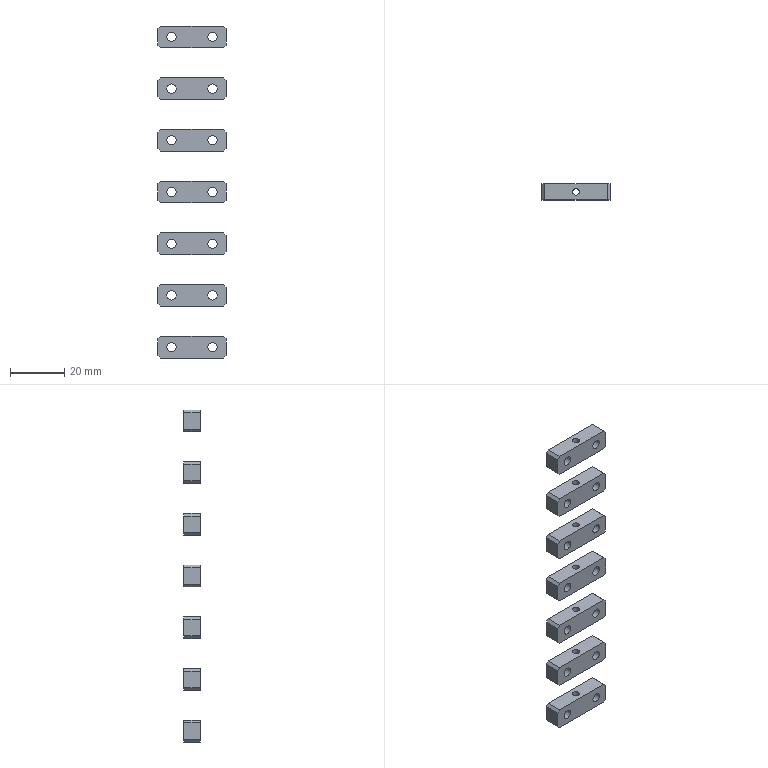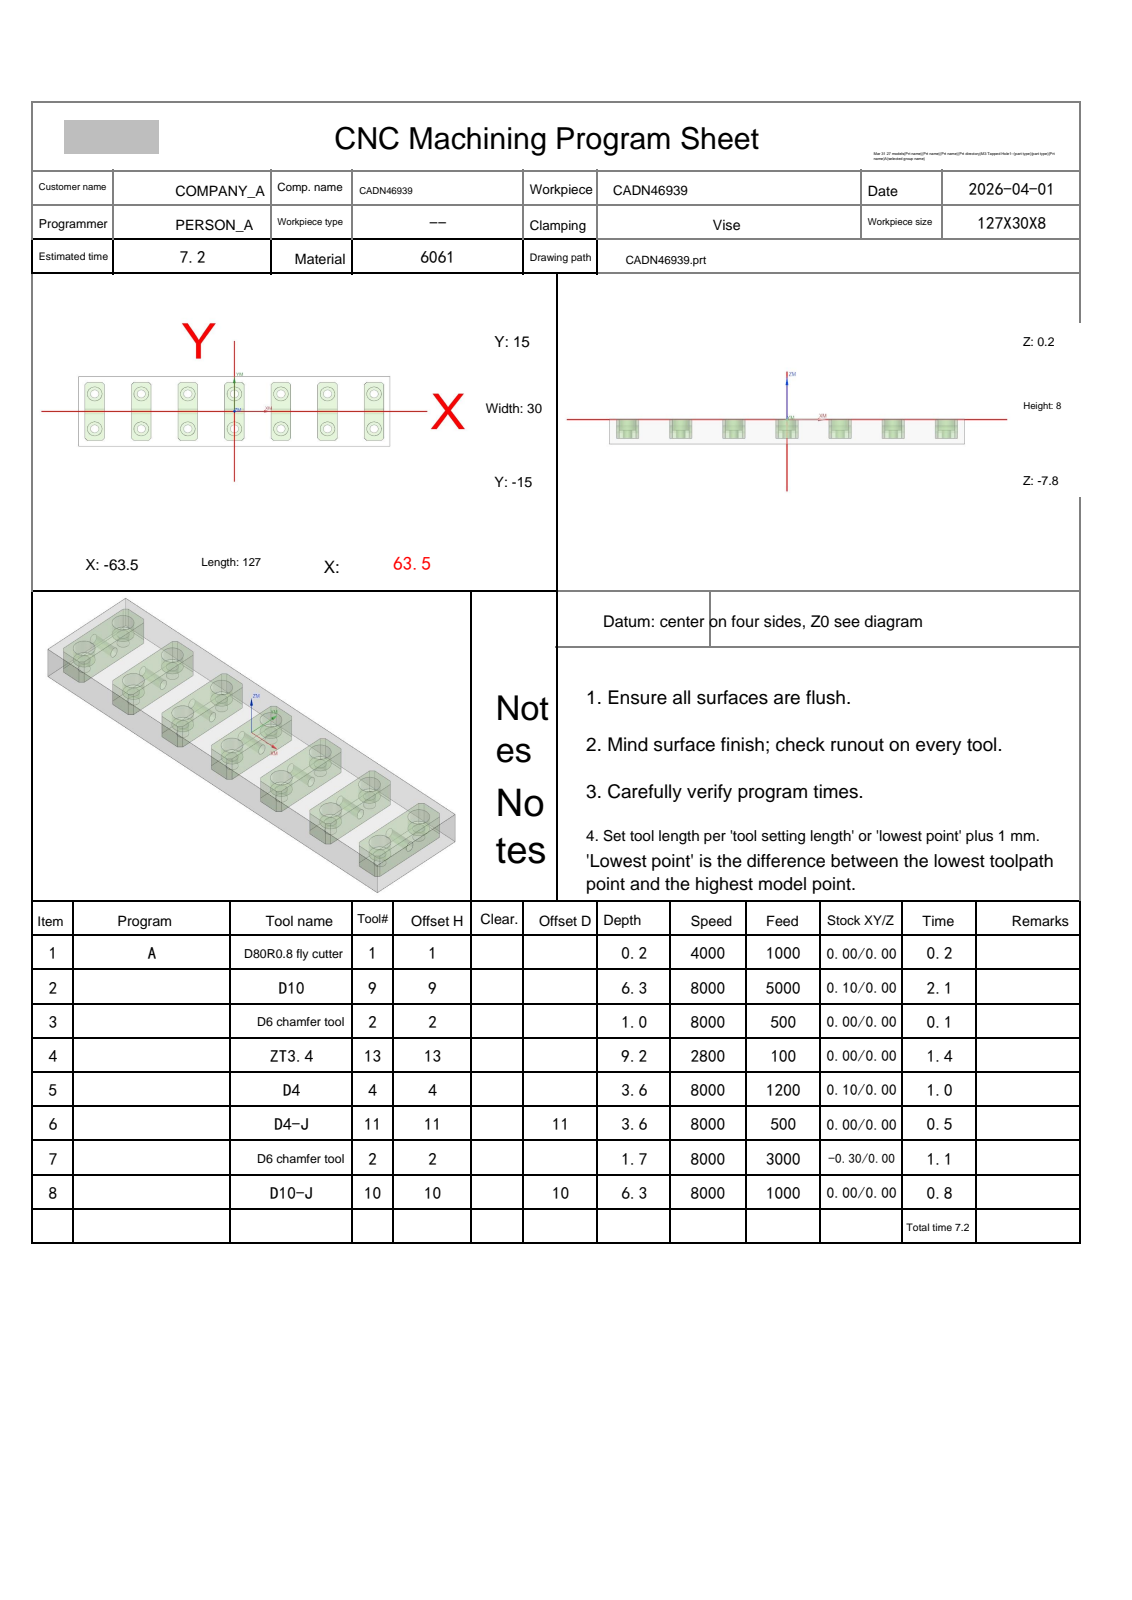NC program | NX | posted by the shop | part box 25 x 6 x 122 mm
Lines 1772 to 3537 of 3537, first 1667 of 1766 lines:
N3 T02 M06
(D6 chamfer tool  D=6. R=0. H=02 ce=0.00 di=0.00)
G00 G90 G54 X-57. Y7.5 M03 S8000
G43 H02 Z20.
M08
G98 G81 X-57. Y7.5 Z-.8 R1. F500.
Y-7.5
X-38.
Y7.5
X-19.
Y-7.5
X0.0
Y7.5
X19.
Y-7.5
X38.
Y7.5
X57.
Y-7.5
G80
G00 Z20.
G91 G28 Z0.0
M05
M09
G91 G28 Z0.0
M01
N4 T13 M06
(ZT3.4 D=3.4 DR_a=118 H=13)
G00 G90 G54 X-57. Y7.5 M03 S2800
G43 H13 Z20.
M08
G98 G83 X-57. Y7.5 Z-9.021 R1. F100. Q2.
Y-7.5
X-38.
Y7.5
X-19.
Y-7.5
X0.0
Y7.5
X19.
Y-7.5
X38.
Y7.5
X57.
Y-7.5
G80
G00 Z20.
G91 G28 Z0.0
M05
M09
G91 G28 Z0.0
M01
N5 T04 M06
(D4  D=4. R=0. H=04 ce=0.10 di=0.00)
G00 G90 G54 X-57. Y7.5 M03 S8000
G43 H04 Z20.
M08
Z.5
G03 X-56.55 Y7.95 I0.0 J.45 F1200.
X-57. Y8.4 I-.45 J0.0
X-57. Y8.4 Z.2 I0.0 J-.9
X-57. Y8.4 Z-.1 I0.0 J-.9
X-57. Y8.4 Z-.4 I0.0 J-.9
X-57. Y8.4 Z-.7 I0.0 J-.9
X-57. Y8.4 Z-1. I0.0 J-.9
X-57. Y8.4 Z-1.3 I0.0 J-.9
X-57. Y8.4 Z-1.6 I0.0 J-.9
X-57. Y8.4 Z-1.9 I0.0 J-.9
X-57. Y8.4 Z-2.2 I0.0 J-.9
X-57. Y8.4 Z-2.5 I0.0 J-.9
X-57. Y8.4 Z-2.8 I0.0 J-.9
X-57. Y8.4 Z-3.1 I0.0 J-.9
X-57. Y8.4 Z-3.4 I0.0 J-.9
X-57.9 Y7.5 I0.0 J-.9
X-57. Y6.6 I.9 J0.0
X-56.1 Y7.5 I0.0 J.9
X-57. Y8.4 I-.9 J0.0
X-57.45 Y7.95 I0.0 J-.45
X-57. Y7.5 I.45 J0.0
G00 Z20.
Y-7.5
Z.5
G03 X-56.55 Y-7.05 I0.0 J.45
X-57. Y-6.6 I-.45 J0.0
X-57. Y-6.6 Z.2 I0.0 J-.9
X-57. Y-6.6 Z-.1 I0.0 J-.9
X-57. Y-6.6 Z-.4 I0.0 J-.9
X-57. Y-6.6 Z-.7 I0.0 J-.9
X-57. Y-6.6 Z-1. I0.0 J-.9
X-57. Y-6.6 Z-1.3 I0.0 J-.9
X-57. Y-6.6 Z-1.6 I0.0 J-.9
X-57. Y-6.6 Z-1.9 I0.0 J-.9
X-57. Y-6.6 Z-2.2 I0.0 J-.9
X-57. Y-6.6 Z-2.5 I0.0 J-.9
X-57. Y-6.6 Z-2.8 I0.0 J-.9
X-57. Y-6.6 Z-3.1 I0.0 J-.9
X-57. Y-6.6 Z-3.4 I0.0 J-.9
X-57.9 Y-7.5 I0.0 J-.9
X-57. Y-8.4 I.9 J0.0
X-56.1 Y-7.5 I0.0 J.9
X-57. Y-6.6 I-.9 J0.0
X-57.45 Y-7.05 I0.0 J-.45
X-57. Y-7.5 I.45 J0.0
G00 Z20.
X-38.
Z.5
G03 X-37.55 Y-7.05 I0.0 J.45
X-38. Y-6.6 I-.45 J0.0
X-38. Y-6.6 Z.2 I0.0 J-.9
X-38. Y-6.6 Z-.1 I0.0 J-.9
X-38. Y-6.6 Z-.4 I0.0 J-.9
X-38. Y-6.6 Z-.7 I0.0 J-.9
X-38. Y-6.6 Z-1. I0.0 J-.9
X-38. Y-6.6 Z-1.3 I0.0 J-.9
X-38. Y-6.6 Z-1.6 I0.0 J-.9
X-38. Y-6.6 Z-1.9 I0.0 J-.9
X-38. Y-6.6 Z-2.2 I0.0 J-.9
X-38. Y-6.6 Z-2.5 I0.0 J-.9
X-38. Y-6.6 Z-2.8 I0.0 J-.9
X-38. Y-6.6 Z-3.1 I0.0 J-.9
X-38. Y-6.6 Z-3.4 I0.0 J-.9
X-38.9 Y-7.5 I0.0 J-.9
X-38. Y-8.4 I.9 J0.0
X-37.1 Y-7.5 I0.0 J.9
X-38. Y-6.6 I-.9 J0.0
X-38.45 Y-7.05 I0.0 J-.45
X-38. Y-7.5 I.45 J0.0
G00 Z20.
Y7.5
Z.5
G03 X-37.55 Y7.95 I0.0 J.45
X-38. Y8.4 I-.45 J0.0
X-38. Y8.4 Z.2 I0.0 J-.9
X-38. Y8.4 Z-.1 I0.0 J-.9
X-38. Y8.4 Z-.4 I0.0 J-.9
X-38. Y8.4 Z-.7 I0.0 J-.9
X-38. Y8.4 Z-1. I0.0 J-.9
X-38. Y8.4 Z-1.3 I0.0 J-.9
X-38. Y8.4 Z-1.6 I0.0 J-.9
X-38. Y8.4 Z-1.9 I0.0 J-.9
X-38. Y8.4 Z-2.2 I0.0 J-.9
X-38. Y8.4 Z-2.5 I0.0 J-.9
X-38. Y8.4 Z-2.8 I0.0 J-.9
X-38. Y8.4 Z-3.1 I0.0 J-.9
X-38. Y8.4 Z-3.4 I0.0 J-.9
X-38.9 Y7.5 I0.0 J-.9
X-38. Y6.6 I.9 J0.0
X-37.1 Y7.5 I0.0 J.9
X-38. Y8.4 I-.9 J0.0
X-38.45 Y7.95 I0.0 J-.45
X-38. Y7.5 I.45 J0.0
G00 Z20.
X-19.
Z.5
G03 X-18.55 Y7.95 I0.0 J.45
X-19. Y8.4 I-.45 J0.0
X-19. Y8.4 Z.2 I0.0 J-.9
X-19. Y8.4 Z-.1 I0.0 J-.9
X-19. Y8.4 Z-.4 I0.0 J-.9
X-19. Y8.4 Z-.7 I0.0 J-.9
X-19. Y8.4 Z-1. I0.0 J-.9
X-19. Y8.4 Z-1.3 I0.0 J-.9
X-19. Y8.4 Z-1.6 I0.0 J-.9
X-19. Y8.4 Z-1.9 I0.0 J-.9
X-19. Y8.4 Z-2.2 I0.0 J-.9
X-19. Y8.4 Z-2.5 I0.0 J-.9
X-19. Y8.4 Z-2.8 I0.0 J-.9
X-19. Y8.4 Z-3.1 I0.0 J-.9
X-19. Y8.4 Z-3.4 I0.0 J-.9
X-19.9 Y7.5 I0.0 J-.9
X-19. Y6.6 I.9 J0.0
X-18.1 Y7.5 I0.0 J.9
X-19. Y8.4 I-.9 J0.0
X-19.45 Y7.95 I0.0 J-.45
X-19. Y7.5 I.45 J0.0
G00 Z20.
Y-7.5
Z.5
G03 X-18.55 Y-7.05 I0.0 J.45
X-19. Y-6.6 I-.45 J0.0
X-19. Y-6.6 Z.2 I0.0 J-.9
X-19. Y-6.6 Z-.1 I0.0 J-.9
X-19. Y-6.6 Z-.4 I0.0 J-.9
X-19. Y-6.6 Z-.7 I0.0 J-.9
X-19. Y-6.6 Z-1. I0.0 J-.9
X-19. Y-6.6 Z-1.3 I0.0 J-.9
X-19. Y-6.6 Z-1.6 I0.0 J-.9
X-19. Y-6.6 Z-1.9 I0.0 J-.9
X-19. Y-6.6 Z-2.2 I0.0 J-.9
X-19. Y-6.6 Z-2.5 I0.0 J-.9
X-19. Y-6.6 Z-2.8 I0.0 J-.9
X-19. Y-6.6 Z-3.1 I0.0 J-.9
X-19. Y-6.6 Z-3.4 I0.0 J-.9
X-19.9 Y-7.5 I0.0 J-.9
X-19. Y-8.4 I.9 J0.0
X-18.1 Y-7.5 I0.0 J.9
X-19. Y-6.6 I-.9 J0.0
X-19.45 Y-7.05 I0.0 J-.45
X-19. Y-7.5 I.45 J0.0
G00 Z20.
X0.0
Z.5
G03 X.45 Y-7.05 I0.0 J.45
X0.0 Y-6.6 I-.45 J0.0
X0.0 Y-6.6 Z.2 I0.0 J-.9
X0.0 Y-6.6 Z-.1 I0.0 J-.9
X0.0 Y-6.6 Z-.4 I0.0 J-.9
X0.0 Y-6.6 Z-.7 I0.0 J-.9
X0.0 Y-6.6 Z-1. I0.0 J-.9
X0.0 Y-6.6 Z-1.3 I0.0 J-.9
X0.0 Y-6.6 Z-1.6 I0.0 J-.9
X0.0 Y-6.6 Z-1.9 I0.0 J-.9
X0.0 Y-6.6 Z-2.2 I0.0 J-.9
X0.0 Y-6.6 Z-2.5 I0.0 J-.9
X0.0 Y-6.6 Z-2.8 I0.0 J-.9
X0.0 Y-6.6 Z-3.1 I0.0 J-.9
X0.0 Y-6.6 Z-3.4 I0.0 J-.9
X-.9 Y-7.5 I0.0 J-.9
X0.0 Y-8.4 I.9 J0.0
X.9 Y-7.5 I0.0 J.9
X0.0 Y-6.6 I-.9 J0.0
X-.45 Y-7.05 I0.0 J-.45
X0.0 Y-7.5 I.45 J0.0
G00 Z20.
Y7.5
Z.5
G03 X.45 Y7.95 I0.0 J.45
X0.0 Y8.4 I-.45 J0.0
X0.0 Y8.4 Z.2 I0.0 J-.9
X0.0 Y8.4 Z-.1 I0.0 J-.9
X0.0 Y8.4 Z-.4 I0.0 J-.9
X0.0 Y8.4 Z-.7 I0.0 J-.9
X0.0 Y8.4 Z-1. I0.0 J-.9
X0.0 Y8.4 Z-1.3 I0.0 J-.9
X0.0 Y8.4 Z-1.6 I0.0 J-.9
X0.0 Y8.4 Z-1.9 I0.0 J-.9
X0.0 Y8.4 Z-2.2 I0.0 J-.9
X0.0 Y8.4 Z-2.5 I0.0 J-.9
X0.0 Y8.4 Z-2.8 I0.0 J-.9
X0.0 Y8.4 Z-3.1 I0.0 J-.9
X0.0 Y8.4 Z-3.4 I0.0 J-.9
X-.9 Y7.5 I0.0 J-.9
X0.0 Y6.6 I.9 J0.0
X.9 Y7.5 I0.0 J.9
X0.0 Y8.4 I-.9 J0.0
X-.45 Y7.95 I0.0 J-.45
X0.0 Y7.5 I.45 J0.0
G00 Z20.
X19.
Z.5
G03 X19.45 Y7.95 I0.0 J.45
X19. Y8.4 I-.45 J0.0
X19. Y8.4 Z.2 I0.0 J-.9
X19. Y8.4 Z-.1 I0.0 J-.9
X19. Y8.4 Z-.4 I0.0 J-.9
X19. Y8.4 Z-.7 I0.0 J-.9
X19. Y8.4 Z-1. I0.0 J-.9
X19. Y8.4 Z-1.3 I0.0 J-.9
X19. Y8.4 Z-1.6 I0.0 J-.9
X19. Y8.4 Z-1.9 I0.0 J-.9
X19. Y8.4 Z-2.2 I0.0 J-.9
X19. Y8.4 Z-2.5 I0.0 J-.9
X19. Y8.4 Z-2.8 I0.0 J-.9
X19. Y8.4 Z-3.1 I0.0 J-.9
X19. Y8.4 Z-3.4 I0.0 J-.9
X18.1 Y7.5 I0.0 J-.9
X19. Y6.6 I.9 J0.0
X19.9 Y7.5 I0.0 J.9
X19. Y8.4 I-.9 J0.0
X18.55 Y7.95 I0.0 J-.45
X19. Y7.5 I.45 J0.0
G00 Z20.
Y-7.5
Z.5
G03 X19.45 Y-7.05 I0.0 J.45
X19. Y-6.6 I-.45 J0.0
X19. Y-6.6 Z.2 I0.0 J-.9
X19. Y-6.6 Z-.1 I0.0 J-.9
X19. Y-6.6 Z-.4 I0.0 J-.9
X19. Y-6.6 Z-.7 I0.0 J-.9
X19. Y-6.6 Z-1. I0.0 J-.9
X19. Y-6.6 Z-1.3 I0.0 J-.9
X19. Y-6.6 Z-1.6 I0.0 J-.9
X19. Y-6.6 Z-1.9 I0.0 J-.9
X19. Y-6.6 Z-2.2 I0.0 J-.9
X19. Y-6.6 Z-2.5 I0.0 J-.9
X19. Y-6.6 Z-2.8 I0.0 J-.9
X19. Y-6.6 Z-3.1 I0.0 J-.9
X19. Y-6.6 Z-3.4 I0.0 J-.9
X18.1 Y-7.5 I0.0 J-.9
X19. Y-8.4 I.9 J0.0
X19.9 Y-7.5 I0.0 J.9
X19. Y-6.6 I-.9 J0.0
X18.55 Y-7.05 I0.0 J-.45
X19. Y-7.5 I.45 J0.0
G00 Z20.
X38.
Z.5
G03 X38.45 Y-7.05 I0.0 J.45
X38. Y-6.6 I-.45 J0.0
X38. Y-6.6 Z.2 I0.0 J-.9
X38. Y-6.6 Z-.1 I0.0 J-.9
X38. Y-6.6 Z-.4 I0.0 J-.9
X38. Y-6.6 Z-.7 I0.0 J-.9
X38. Y-6.6 Z-1. I0.0 J-.9
X38. Y-6.6 Z-1.3 I0.0 J-.9
X38. Y-6.6 Z-1.6 I0.0 J-.9
X38. Y-6.6 Z-1.9 I0.0 J-.9
X38. Y-6.6 Z-2.2 I0.0 J-.9
X38. Y-6.6 Z-2.5 I0.0 J-.9
X38. Y-6.6 Z-2.8 I0.0 J-.9
X38. Y-6.6 Z-3.1 I0.0 J-.9
X38. Y-6.6 Z-3.4 I0.0 J-.9
X37.1 Y-7.5 I0.0 J-.9
X38. Y-8.4 I.9 J0.0
X38.9 Y-7.5 I0.0 J.9
X38. Y-6.6 I-.9 J0.0
X37.55 Y-7.05 I0.0 J-.45
X38. Y-7.5 I.45 J0.0
G00 Z20.
Y7.5
Z.5
G03 X38.45 Y7.95 I0.0 J.45
X38. Y8.4 I-.45 J0.0
X38. Y8.4 Z.2 I0.0 J-.9
X38. Y8.4 Z-.1 I0.0 J-.9
X38. Y8.4 Z-.4 I0.0 J-.9
X38. Y8.4 Z-.7 I0.0 J-.9
X38. Y8.4 Z-1. I0.0 J-.9
X38. Y8.4 Z-1.3 I0.0 J-.9
X38. Y8.4 Z-1.6 I0.0 J-.9
X38. Y8.4 Z-1.9 I0.0 J-.9
X38. Y8.4 Z-2.2 I0.0 J-.9
X38. Y8.4 Z-2.5 I0.0 J-.9
X38. Y8.4 Z-2.8 I0.0 J-.9
X38. Y8.4 Z-3.1 I0.0 J-.9
X38. Y8.4 Z-3.4 I0.0 J-.9
X37.1 Y7.5 I0.0 J-.9
X38. Y6.6 I.9 J0.0
X38.9 Y7.5 I0.0 J.9
X38. Y8.4 I-.9 J0.0
X37.55 Y7.95 I0.0 J-.45
X38. Y7.5 I.45 J0.0
G00 Z20.
X57.
Z.5
G03 X57.45 Y7.95 I0.0 J.45
X57. Y8.4 I-.45 J0.0
X57. Y8.4 Z.2 I0.0 J-.9
X57. Y8.4 Z-.1 I0.0 J-.9
X57. Y8.4 Z-.4 I0.0 J-.9
X57. Y8.4 Z-.7 I0.0 J-.9
X57. Y8.4 Z-1. I0.0 J-.9
X57. Y8.4 Z-1.3 I0.0 J-.9
X57. Y8.4 Z-1.6 I0.0 J-.9
X57. Y8.4 Z-1.9 I0.0 J-.9
X57. Y8.4 Z-2.2 I0.0 J-.9
X57. Y8.4 Z-2.5 I0.0 J-.9
X57. Y8.4 Z-2.8 I0.0 J-.9
X57. Y8.4 Z-3.1 I0.0 J-.9
X57. Y8.4 Z-3.4 I0.0 J-.9
X56.1 Y7.5 I0.0 J-.9
X57. Y6.6 I.9 J0.0
X57.9 Y7.5 I0.0 J.9
X57. Y8.4 I-.9 J0.0
X56.55 Y7.95 I0.0 J-.45
X57. Y7.5 I.45 J0.0
G00 Z20.
Y-7.5
Z.5
G03 X57.45 Y-7.05 I0.0 J.45
X57. Y-6.6 I-.45 J0.0
X57. Y-6.6 Z.2 I0.0 J-.9
X57. Y-6.6 Z-.1 I0.0 J-.9
X57. Y-6.6 Z-.4 I0.0 J-.9
X57. Y-6.6 Z-.7 I0.0 J-.9
X57. Y-6.6 Z-1. I0.0 J-.9
X57. Y-6.6 Z-1.3 I0.0 J-.9
X57. Y-6.6 Z-1.6 I0.0 J-.9
X57. Y-6.6 Z-1.9 I0.0 J-.9
X57. Y-6.6 Z-2.2 I0.0 J-.9
X57. Y-6.6 Z-2.5 I0.0 J-.9
X57. Y-6.6 Z-2.8 I0.0 J-.9
X57. Y-6.6 Z-3.1 I0.0 J-.9
X57. Y-6.6 Z-3.4 I0.0 J-.9
X56.1 Y-7.5 I0.0 J-.9
X57. Y-8.4 I.9 J0.0
X57.9 Y-7.5 I0.0 J.9
X57. Y-6.6 I-.9 J0.0
X56.55 Y-7.05 I0.0 J-.45
X57. Y-7.5 I.45 J0.0
G00 Z20.
G91 G28 Z0.0
M05
M09
G91 G28 Z0.0
M01
N6 T11 M06
(D4-J  D=4. R=0. H=11 ce=0.00 di=0.00)
G00 G90 G54 X-57. Y7.5 M03 S8000
G43 H11 Z20.
M08
Z.5
G41 D11
G01 X-56.815 Y7.577 F500.
G03 X-56.52 Y8.02 I-.185 J.443
X-57. Y8.5 I-.48 J0.0
X-56.018 Y7.687 Z-3.4 I0.0 J-1.
X-57. Y8.5 I-.982 J-.187
X-58. Y7.5 I0.0 J-1.
X-57. Y6.5 I1. J0.0
X-56. Y7.5 I0.0 J1.
G01 X-56.018 Y7.687
G03 X-56.489 Y8.077 I-.471 J-.09
X-56.959 Y7.696 I0.0 J-.48
G01 G40 X-57. Y7.5
G00 Z20.
Y-7.5
Z.5
G41 D11
G01 X-56.815 Y-7.423
G03 X-56.52 Y-6.98 I-.185 J.443
X-57. Y-6.5 I-.48 J0.0
X-56.018 Y-7.313 Z-3.4 I0.0 J-1.
X-57. Y-6.5 I-.982 J-.187
X-58. Y-7.5 I0.0 J-1.
X-57. Y-8.5 I1. J0.0
X-56. Y-7.5 I0.0 J1.
G01 X-56.018 Y-7.313
G03 X-56.489 Y-6.923 I-.471 J-.09
X-56.959 Y-7.304 I0.0 J-.48
G01 G40 X-57. Y-7.5
G00 Z20.
X-38.
Z.5
G41 D11
G01 X-37.815 Y-7.423
G03 X-37.52 Y-6.98 I-.185 J.443
X-38. Y-6.5 I-.48 J0.0
X-37.018 Y-7.313 Z-3.4 I0.0 J-1.
X-38. Y-6.5 I-.982 J-.187
X-39. Y-7.5 I0.0 J-1.
X-38. Y-8.5 I1. J0.0
X-37. Y-7.5 I0.0 J1.
G01 X-37.018 Y-7.313
G03 X-37.489 Y-6.923 I-.471 J-.09
X-37.959 Y-7.304 I0.0 J-.48
G01 G40 X-38. Y-7.5
G00 Z20.
Y7.5
Z.5
G41 D11
G01 X-37.815 Y7.577
G03 X-37.52 Y8.02 I-.185 J.443
X-38. Y8.5 I-.48 J0.0
X-37.018 Y7.687 Z-3.4 I0.0 J-1.
X-38. Y8.5 I-.982 J-.187
X-39. Y7.5 I0.0 J-1.
X-38. Y6.5 I1. J0.0
X-37. Y7.5 I0.0 J1.
G01 X-37.018 Y7.687
G03 X-37.489 Y8.077 I-.471 J-.09
X-37.959 Y7.696 I0.0 J-.48
G01 G40 X-38. Y7.5
G00 Z20.
X-19.
Z.5
G41 D11
G01 X-18.815 Y7.577
G03 X-18.52 Y8.02 I-.185 J.443
X-19. Y8.5 I-.48 J0.0
X-18.018 Y7.687 Z-3.4 I0.0 J-1.
X-19. Y8.5 I-.982 J-.187
X-20. Y7.5 I0.0 J-1.
X-19. Y6.5 I1. J0.0
X-18. Y7.5 I0.0 J1.
G01 X-18.018 Y7.687
G03 X-18.489 Y8.077 I-.471 J-.09
X-18.959 Y7.696 I0.0 J-.48
G01 G40 X-19. Y7.5
G00 Z20.
Y-7.5
Z.5
G41 D11
G01 X-18.815 Y-7.423
G03 X-18.52 Y-6.98 I-.185 J.443
X-19. Y-6.5 I-.48 J0.0
X-18.018 Y-7.313 Z-3.4 I0.0 J-1.
X-19. Y-6.5 I-.982 J-.187
X-20. Y-7.5 I0.0 J-1.
X-19. Y-8.5 I1. J0.0
X-18. Y-7.5 I0.0 J1.
G01 X-18.018 Y-7.313
G03 X-18.489 Y-6.923 I-.471 J-.09
X-18.959 Y-7.304 I0.0 J-.48
G01 G40 X-19. Y-7.5
G00 Z20.
X0.0
Z.5
G41 D11
G01 X.185 Y-7.423
G03 X.48 Y-6.98 I-.185 J.443
X0.0 Y-6.5 I-.48 J0.0
X.982 Y-7.313 Z-3.4 I0.0 J-1.
X0.0 Y-6.5 I-.982 J-.187
X-1. Y-7.5 I0.0 J-1.
X0.0 Y-8.5 I1. J0.0
X1. Y-7.5 I0.0 J1.
G01 X.982 Y-7.313
G03 X.511 Y-6.923 I-.471 J-.09
X.041 Y-7.304 I0.0 J-.48
G01 G40 X0.0 Y-7.5
G00 Z20.
Y7.5
Z.5
G41 D11
G01 X.185 Y7.577
G03 X.48 Y8.02 I-.185 J.443
X0.0 Y8.5 I-.48 J0.0
X.982 Y7.687 Z-3.4 I0.0 J-1.
X0.0 Y8.5 I-.982 J-.187
X-1. Y7.5 I0.0 J-1.
X0.0 Y6.5 I1. J0.0
X1. Y7.5 I0.0 J1.
G01 X.982 Y7.687
G03 X.511 Y8.077 I-.471 J-.09
X.041 Y7.696 I0.0 J-.48
G01 G40 X0.0 Y7.5
G00 Z20.
X19.
Z.5
G41 D11
G01 X19.185 Y7.577
G03 X19.48 Y8.02 I-.185 J.443
X19. Y8.5 I-.48 J0.0
X19.982 Y7.687 Z-3.4 I0.0 J-1.
X19. Y8.5 I-.982 J-.187
X18. Y7.5 I0.0 J-1.
X19. Y6.5 I1. J0.0
X20. Y7.5 I0.0 J1.
G01 X19.982 Y7.687
G03 X19.511 Y8.077 I-.471 J-.09
X19.041 Y7.696 I0.0 J-.48
G01 G40 X19. Y7.5
G00 Z20.
Y-7.5
Z.5
G41 D11
G01 X19.185 Y-7.423
G03 X19.48 Y-6.98 I-.185 J.443
X19. Y-6.5 I-.48 J0.0
X19.982 Y-7.313 Z-3.4 I0.0 J-1.
X19. Y-6.5 I-.982 J-.187
X18. Y-7.5 I0.0 J-1.
X19. Y-8.5 I1. J0.0
X20. Y-7.5 I0.0 J1.
G01 X19.982 Y-7.313
G03 X19.511 Y-6.923 I-.471 J-.09
X19.041 Y-7.304 I0.0 J-.48
G01 G40 X19. Y-7.5
G00 Z20.
X38.
Z.5
G41 D11
G01 X38.185 Y-7.423
G03 X38.48 Y-6.98 I-.185 J.443
X38. Y-6.5 I-.48 J0.0
X38.982 Y-7.313 Z-3.4 I0.0 J-1.
X38. Y-6.5 I-.982 J-.187
X37. Y-7.5 I0.0 J-1.
X38. Y-8.5 I1. J0.0
X39. Y-7.5 I0.0 J1.
G01 X38.982 Y-7.313
G03 X38.511 Y-6.923 I-.471 J-.09
X38.041 Y-7.304 I0.0 J-.48
G01 G40 X38. Y-7.5
G00 Z20.
Y7.5
Z.5
G41 D11
G01 X38.185 Y7.577
G03 X38.48 Y8.02 I-.185 J.443
X38. Y8.5 I-.48 J0.0
X38.982 Y7.687 Z-3.4 I0.0 J-1.
X38. Y8.5 I-.982 J-.187
X37. Y7.5 I0.0 J-1.
X38. Y6.5 I1. J0.0
X39. Y7.5 I0.0 J1.
G01 X38.982 Y7.687
G03 X38.511 Y8.077 I-.471 J-.09
X38.041 Y7.696 I0.0 J-.48
G01 G40 X38. Y7.5
G00 Z20.
X57.
Z.5
G41 D11
G01 X57.185 Y7.577
G03 X57.48 Y8.02 I-.185 J.443
X57. Y8.5 I-.48 J0.0
X57.982 Y7.687 Z-3.4 I0.0 J-1.
X57. Y8.5 I-.982 J-.187
X56. Y7.5 I0.0 J-1.
X57. Y6.5 I1. J0.0
X58. Y7.5 I0.0 J1.
G01 X57.982 Y7.687
G03 X57.511 Y8.077 I-.471 J-.09
X57.041 Y7.696 I0.0 J-.48
G01 G40 X57. Y7.5
G00 Z20.
Y-7.5
Z.5
G41 D11
G01 X57.185 Y-7.423
G03 X57.48 Y-6.98 I-.185 J.443
X57. Y-6.5 I-.48 J0.0
X57.982 Y-7.313 Z-3.4 I0.0 J-1.
X57. Y-6.5 I-.982 J-.187
X56. Y-7.5 I0.0 J-1.
X57. Y-8.5 I1. J0.0
X58. Y-7.5 I0.0 J1.
G01 X57.982 Y-7.313
G03 X57.511 Y-6.923 I-.471 J-.09
X57.041 Y-7.304 I0.0 J-.48
G01 G40 X57. Y-7.5
G00 Z20.
G91 G28 Z0.0
M05
M09
G91 G28 Z0.0
M01
N7 T02 M06
(D6 chamfer tool  D=6. R=0. H=02 ce=0.00 di=0.00)
G00 G90 G54 X63.128 Y.25 M03 S8000
G43 H02 Z20.
M08
Z2.099
G01 Z-1.5 F3000.
G03 X62.828 Y.33 I-.3 J-.52
X62.308 Y.03 I0.0 J-.6
G01 X62.3 Y0.0
Y-11.5
X62.275 Y-11.754
X62.201 Y-11.997
X62.081 Y-12.222
X61.919 Y-12.419
X60.919 Y-13.419
X60.722 Y-13.581
X60.497 Y-13.701
X60.254 Y-13.775
X60. Y-13.8
X54.
X53.746 Y-13.775
X53.503 Y-13.701
X53.278 Y-13.581
X53.081 Y-13.419
X52.081 Y-12.419
X51.919 Y-12.222
X51.799 Y-11.997
X51.725 Y-11.754
X51.7 Y-11.5
Y11.5
X51.725 Y11.754
X51.799 Y11.997
X51.919 Y12.222
X52.081 Y12.419
X53.081 Y13.419
X53.278 Y13.581
X53.503 Y13.701
X53.746 Y13.775
X54. Y13.8
X60.
X60.254 Y13.775
X60.497 Y13.701
X60.722 Y13.581
X60.919 Y13.419
X61.919 Y12.419
X62.081 Y12.222
X62.201 Y11.997
X62.275 Y11.754
X62.3 Y11.5
Y0.0
X62.308 Y-.03
G03 X62.828 Y-.33 I.52 J.3
X63.128 Y-.25 I0.0 J.6
G01 Z2.099
G00 Z20.
X31.872
Z2.099
G01 Z-1.5
G03 X32.172 Y-.33 I.3 J.52
X32.692 Y-.03 I0.0 J.6
G01 X32.7 Y0.0
Y11.5
X32.725 Y11.754
X32.799 Y11.997
X32.919 Y12.222
X33.081 Y12.419
X34.081 Y13.419
X34.278 Y13.581
X34.503 Y13.701
X34.746 Y13.775
X35. Y13.8
X41.
X41.254 Y13.775
X41.497 Y13.701
X41.722 Y13.581
X41.919 Y13.419
X42.919 Y12.419
X43.081 Y12.222
X43.201 Y11.997
X43.275 Y11.754
X43.3 Y11.5
Y-11.5
X43.275 Y-11.754
X43.201 Y-11.997
X43.081 Y-12.222
X42.919 Y-12.419
X41.919 Y-13.419
X41.722 Y-13.581
X41.497 Y-13.701
X41.254 Y-13.775
X41. Y-13.8
X35.
X34.746 Y-13.775
X34.503 Y-13.701
X34.278 Y-13.581
X34.081 Y-13.419
X33.081 Y-12.419
X32.919 Y-12.222
X32.799 Y-11.997
X32.725 Y-11.754
X32.7 Y-11.5
Y0.0
X32.692 Y.03
G03 X32.172 Y.33 I-.52 J-.3
X31.872 Y.25 I0.0 J-.6
G01 Z2.099
G00 Z20.
X12.872 Y-.25
Z2.099
G01 Z-1.5
G03 X13.172 Y-.33 I.3 J.52
X13.692 Y-.03 I0.0 J.6
G01 X13.7 Y0.0
Y11.5
X13.725 Y11.754
X13.799 Y11.997
X13.919 Y12.222
X14.081 Y12.419
X15.081 Y13.419
X15.278 Y13.581
X15.503 Y13.701
X15.746 Y13.775
X16. Y13.8
X22.
X22.254 Y13.775
X22.497 Y13.701
X22.722 Y13.581
X22.919 Y13.419
X23.919 Y12.419
X24.081 Y12.222
X24.201 Y11.997
X24.275 Y11.754
X24.3 Y11.5
Y-11.5
X24.275 Y-11.754
X24.201 Y-11.997
X24.081 Y-12.222
X23.919 Y-12.419
X22.919 Y-13.419
X22.722 Y-13.581
X22.497 Y-13.701
X22.254 Y-13.775
X22. Y-13.8
X16.
X15.746 Y-13.775
X15.503 Y-13.701
X15.278 Y-13.581
X15.081 Y-13.419
X14.081 Y-12.419
X13.919 Y-12.222
X13.799 Y-11.997
X13.725 Y-11.754
X13.7 Y-11.5
Y0.0
X13.692 Y.03
G03 X13.172 Y.33 I-.52 J-.3
X12.872 Y.25 I0.0 J-.6
G01 Z2.099
G00 Z20.
X-6.128 Y-.25
Z2.099
G01 Z-1.5
G03 X-5.828 Y-.33 I.3 J.52
X-5.308 Y-.03 I0.0 J.6
G01 X-5.3 Y0.0
Y11.5
X-5.275 Y11.754
X-5.201 Y11.997
X-5.081 Y12.222
X-4.919 Y12.419
X-3.919 Y13.419
X-3.722 Y13.581
X-3.497 Y13.701
X-3.254 Y13.775
X-3. Y13.8
X3.
X3.254 Y13.775
X3.497 Y13.701
X3.722 Y13.581
X3.919 Y13.419
X4.919 Y12.419
X5.081 Y12.222
X5.201 Y11.997
X5.275 Y11.754
X5.3 Y11.5
Y-11.5
X5.275 Y-11.754
X5.201 Y-11.997
X5.081 Y-12.222
X4.919 Y-12.419
X3.919 Y-13.419
X3.722 Y-13.581
X3.497 Y-13.701
X3.254 Y-13.775
X3. Y-13.8
X-3.
X-3.254 Y-13.775
X-3.497 Y-13.701
X-3.722 Y-13.581
X-3.919 Y-13.419
X-4.919 Y-12.419
X-5.081 Y-12.222
X-5.201 Y-11.997
X-5.275 Y-11.754
X-5.3 Y-11.5
Y0.0
X-5.308 Y.03
G03 X-5.828 Y.33 I-.52 J-.3
X-6.128 Y.25 I0.0 J-.6
G01 Z2.099
G00 Z20.
X-25.128 Y-.25
Z2.099
G01 Z-1.5
G03 X-24.828 Y-.33 I.3 J.52
X-24.308 Y-.03 I0.0 J.6
G01 X-24.3 Y0.0
Y11.5
X-24.275 Y11.754
X-24.201 Y11.997
X-24.081 Y12.222
X-23.919 Y12.419
X-22.919 Y13.419
X-22.722 Y13.581
X-22.497 Y13.701
X-22.254 Y13.775
X-22. Y13.8
X-16.
X-15.746 Y13.775
X-15.503 Y13.701
X-15.278 Y13.581
X-15.081 Y13.419
X-14.081 Y12.419
X-13.919 Y12.222
X-13.799 Y11.997
X-13.725 Y11.754
X-13.7 Y11.5
Y-11.5
X-13.725 Y-11.754
X-13.799 Y-11.997
X-13.919 Y-12.222
X-14.081 Y-12.419
X-15.081 Y-13.419
X-15.278 Y-13.581
X-15.503 Y-13.701
X-15.746 Y-13.775
X-16. Y-13.8
X-22.
X-22.254 Y-13.775
X-22.497 Y-13.701
X-22.722 Y-13.581
X-22.919 Y-13.419
X-23.919 Y-12.419
X-24.081 Y-12.222
X-24.201 Y-11.997
X-24.275 Y-11.754
X-24.3 Y-11.5
Y0.0
X-24.308 Y.03
G03 X-24.828 Y.33 I-.52 J-.3
X-25.128 Y.25 I0.0 J-.6
G01 Z2.099
G00 Z20.
X-44.128 Y-.25
Z2.099
G01 Z-1.5
G03 X-43.828 Y-.33 I.3 J.52
X-43.308 Y-.03 I0.0 J.6
G01 X-43.3 Y0.0
Y11.5
X-43.275 Y11.754
X-43.201 Y11.997
X-43.081 Y12.222
X-42.919 Y12.419
X-41.919 Y13.419
X-41.722 Y13.581
X-41.497 Y13.701
X-41.254 Y13.775
X-41. Y13.8
X-35.
X-34.746 Y13.775
X-34.503 Y13.701
X-34.278 Y13.581
X-34.081 Y13.419
X-33.081 Y12.419
X-32.919 Y12.222
X-32.799 Y11.997
X-32.725 Y11.754
X-32.7 Y11.5
Y-11.5
X-32.725 Y-11.754
X-32.799 Y-11.997
X-32.919 Y-12.222
X-33.081 Y-12.419
X-34.081 Y-13.419
X-34.278 Y-13.581
X-34.503 Y-13.701
X-34.746 Y-13.775
X-35. Y-13.8
X-41.
X-41.254 Y-13.775
X-41.497 Y-13.701
X-41.722 Y-13.581
X-41.919 Y-13.419
X-42.919 Y-12.419
X-43.081 Y-12.222
X-43.201 Y-11.997
X-43.275 Y-11.754
X-43.3 Y-11.5
Y0.0
X-43.308 Y.03
G03 X-43.828 Y.33 I-.52 J-.3
X-44.128 Y.25 I0.0 J-.6
G01 Z2.099
G00 Z20.
X-63.128 Y-.25
Z2.099
G01 Z-1.5
G03 X-62.828 Y-.33 I.3 J.52
X-62.308 Y-.03 I0.0 J.6
G01 X-62.3 Y0.0
Y11.5
X-62.275 Y11.754
X-62.201 Y11.997
X-62.081 Y12.222
X-61.919 Y12.419
X-60.919 Y13.419
X-60.722 Y13.581
X-60.497 Y13.701
X-60.254 Y13.775
X-60. Y13.8
X-54.
X-53.746 Y13.775
X-53.503 Y13.701
X-53.278 Y13.581
X-53.081 Y13.419
X-52.081 Y12.419
X-51.919 Y12.222
X-51.799 Y11.997
X-51.725 Y11.754
X-51.7 Y11.5
Y-11.5
X-51.725 Y-11.754
X-51.799 Y-11.997
X-51.919 Y-12.222
X-52.081 Y-12.419
X-53.081 Y-13.419
X-53.278 Y-13.581
X-53.503 Y-13.701
X-53.746 Y-13.775
X-54. Y-13.8
X-60.
X-60.254 Y-13.775
X-60.497 Y-13.701
X-60.722 Y-13.581
X-60.919 Y-13.419
X-61.919 Y-12.419
X-62.081 Y-12.222
X-62.201 Y-11.997
X-62.275 Y-11.754
X-62.3 Y-11.5
Y0.0
X-62.308 Y.03
G03 X-62.828 Y.33 I-.52 J-.3
X-63.128 Y.25 I0.0 J-.6
G01 Z2.099
G00 Z20.
G00 G90 X-55.83 Y5.519 M03 S8000
Z20.
Z2.5
G01 X-55.748 Y5.567 Z2.465 F500.
X-55.487 Y5.764 Z2.346
X-55.256 Y5.996 Z2.227
X-55.06 Y6.259 Z2.108
X-54.904 Y6.546 Z1.989
X-54.79 Y6.853 Z1.87
X-54.72 Y7.173 Z1.75
X-54.697 Y7.5 Z1.631
X-54.72 Y7.827 Z1.512
X-54.79 Y8.147 Z1.393
X-54.904 Y8.454 Z1.274
X-55.06 Y8.741 Z1.154
X-55.256 Y9.004 Z1.035
X-55.487 Y9.236 Z.916
X-55.748 Y9.433 Z.797
X-55.952 Y9.551 Z.711
X-56.253 Y9.679 Z.592
X-56.57 Y9.762 Z.473
X-56.895 Y9.801 Z.354
X-57.222 Y9.792 Z.235
X-57.545 Y9.738 Z.115
X-57.857 Y9.638 Z-.004
X-58.152 Y9.494 Z-.123
X-58.423 Y9.311 Z-.242
X-58.665 Y9.091 Z-.361
X-58.874 Y8.839 Z-.48
X-59.045 Y8.559 Z-.6
X-59.174 Y8.259 Z-.719
X-59.26 Y7.943 Z-.838
X-59.3 Y7.618 Z-.957
Y7.5 Z-1.
G03 X-57. Y5.2 I2.3 J0.0
X-54.7 Y7.5 I0.0 J2.3
X-57. Y9.8 I-2.3 J0.0
X-59.3 Y7.5 I0.0 J-2.3
X-59.246 Y7.004 I2.3 J0.0
G01 Z1.5
G00 Z20.
X-55.83 Y-9.481
Z2.5
G01 X-55.748 Y-9.433 Z2.465
X-55.487 Y-9.236 Z2.346
X-55.256 Y-9.004 Z2.227
X-55.06 Y-8.741 Z2.108
X-54.904 Y-8.454 Z1.989
X-54.79 Y-8.147 Z1.87
X-54.72 Y-7.827 Z1.75
X-54.697 Y-7.5 Z1.631
X-54.72 Y-7.173 Z1.512
X-54.79 Y-6.853 Z1.393
X-54.904 Y-6.546 Z1.274
X-55.06 Y-6.259 Z1.154
X-55.256 Y-5.996 Z1.035
X-55.487 Y-5.764 Z.916
X-55.748 Y-5.567 Z.797
X-55.952 Y-5.449 Z.711
X-56.253 Y-5.321 Z.592
X-56.57 Y-5.238 Z.473
X-56.895 Y-5.199 Z.354
X-57.222 Y-5.208 Z.235
X-57.545 Y-5.262 Z.115
X-57.857 Y-5.362 Z-.004
X-58.152 Y-5.506 Z-.123
X-58.423 Y-5.689 Z-.242
X-58.665 Y-5.909 Z-.361
X-58.874 Y-6.161 Z-.48
X-59.045 Y-6.441 Z-.6
X-59.174 Y-6.741 Z-.719
X-59.26 Y-7.057 Z-.838
X-59.3 Y-7.382 Z-.957
Y-7.5 Z-1.
G03 X-57. Y-9.8 I2.3 J0.0
X-54.7 Y-7.5 I0.0 J2.3
X-57. Y-5.2 I-2.3 J0.0
X-59.3 Y-7.5 I0.0 J-2.3
X-59.246 Y-7.996 I2.3 J0.0
G01 Z1.5
G00 Z20.
X-36.83 Y-9.481
Z2.5
G01 X-36.748 Y-9.433 Z2.465
X-36.487 Y-9.236 Z2.346
X-36.256 Y-9.004 Z2.227
X-36.06 Y-8.741 Z2.108
X-35.904 Y-8.454 Z1.989
X-35.79 Y-8.147 Z1.87
X-35.72 Y-7.827 Z1.75
X-35.697 Y-7.5 Z1.631
X-35.72 Y-7.173 Z1.512
X-35.79 Y-6.853 Z1.393
X-35.904 Y-6.546 Z1.274
X-36.06 Y-6.259 Z1.154
X-36.256 Y-5.996 Z1.035
X-36.487 Y-5.764 Z.916
X-36.748 Y-5.567 Z.797
X-36.952 Y-5.449 Z.711
X-37.253 Y-5.321 Z.592
X-37.57 Y-5.238 Z.473
X-37.895 Y-5.199 Z.354
X-38.222 Y-5.208 Z.235
X-38.545 Y-5.262 Z.115
X-38.857 Y-5.362 Z-.004
X-39.152 Y-5.506 Z-.123
X-39.423 Y-5.689 Z-.242
X-39.665 Y-5.909 Z-.361
X-39.874 Y-6.161 Z-.48
X-40.045 Y-6.441 Z-.6
X-40.174 Y-6.741 Z-.719
X-40.26 Y-7.057 Z-.838
X-40.3 Y-7.382 Z-.957
Y-7.5 Z-1.
G03 X-38. Y-9.8 I2.3 J0.0
X-35.7 Y-7.5 I0.0 J2.3
X-38. Y-5.2 I-2.3 J0.0
X-40.3 Y-7.5 I0.0 J-2.3
X-40.246 Y-7.996 I2.3 J0.0
G01 Z1.5
G00 Z20.
X-36.83 Y5.519
Z2.5
G01 X-36.748 Y5.567 Z2.465
X-36.487 Y5.764 Z2.346
X-36.256 Y5.996 Z2.227
X-36.06 Y6.259 Z2.108
X-35.904 Y6.546 Z1.989
X-35.79 Y6.853 Z1.87
X-35.72 Y7.173 Z1.75
X-35.697 Y7.5 Z1.631
X-35.72 Y7.827 Z1.512
X-35.79 Y8.147 Z1.393
X-35.904 Y8.454 Z1.274
X-36.06 Y8.741 Z1.154
X-36.256 Y9.004 Z1.035
X-36.487 Y9.236 Z.916
X-36.748 Y9.433 Z.797
X-36.952 Y9.551 Z.711
X-37.253 Y9.679 Z.592
X-37.57 Y9.762 Z.473
X-37.895 Y9.801 Z.354
X-38.222 Y9.792 Z.235
X-38.545 Y9.738 Z.115
X-38.857 Y9.638 Z-.004
X-39.152 Y9.494 Z-.123
X-39.423 Y9.311 Z-.242
X-39.665 Y9.091 Z-.361
X-39.874 Y8.839 Z-.48
X-40.045 Y8.559 Z-.6
X-40.174 Y8.259 Z-.719
X-40.26 Y7.943 Z-.838
X-40.3 Y7.618 Z-.957
Y7.5 Z-1.
G03 X-38. Y5.2 I2.3 J0.0
X-35.7 Y7.5 I0.0 J2.3
X-38. Y9.8 I-2.3 J0.0
X-40.3 Y7.5 I0.0 J-2.3
X-40.246 Y7.004 I2.3 J0.0
G01 Z1.5
G00 Z20.
X-17.83 Y5.519
Z2.5
G01 X-17.748 Y5.567 Z2.465
X-17.487 Y5.764 Z2.346
X-17.256 Y5.996 Z2.227
X-17.06 Y6.259 Z2.108
X-16.904 Y6.546 Z1.989
X-16.79 Y6.853 Z1.87
X-16.72 Y7.173 Z1.75
X-16.697 Y7.5 Z1.631
X-16.72 Y7.827 Z1.512
X-16.79 Y8.147 Z1.393
X-16.904 Y8.454 Z1.274
X-17.06 Y8.741 Z1.154
X-17.256 Y9.004 Z1.035
X-17.487 Y9.236 Z.916
X-17.748 Y9.433 Z.797
X-17.952 Y9.551 Z.711
X-18.253 Y9.679 Z.592
X-18.57 Y9.762 Z.473
X-18.895 Y9.801 Z.354
X-19.222 Y9.792 Z.235
X-19.545 Y9.738 Z.115
X-19.857 Y9.638 Z-.004
X-20.152 Y9.494 Z-.123
X-20.423 Y9.311 Z-.242
X-20.665 Y9.091 Z-.361
X-20.874 Y8.839 Z-.48
X-21.045 Y8.559 Z-.6
X-21.174 Y8.259 Z-.719
X-21.26 Y7.943 Z-.838
X-21.3 Y7.618 Z-.957
Y7.5 Z-1.
G03 X-19. Y5.2 I2.3 J0.0
X-16.7 Y7.5 I0.0 J2.3
X-19. Y9.8 I-2.3 J0.0
X-21.3 Y7.5 I0.0 J-2.3
X-21.246 Y7.004 I2.3 J0.0
G01 Z1.5
G00 Z20.
X-17.83 Y-9.481
Z2.5
G01 X-17.748 Y-9.433 Z2.465
X-17.487 Y-9.236 Z2.346
X-17.256 Y-9.004 Z2.227
X-17.06 Y-8.741 Z2.108
X-16.904 Y-8.454 Z1.989
X-16.79 Y-8.147 Z1.87
X-16.72 Y-7.827 Z1.75
X-16.697 Y-7.5 Z1.631
X-16.72 Y-7.173 Z1.512
X-16.79 Y-6.853 Z1.393
X-16.904 Y-6.546 Z1.274
X-17.06 Y-6.259 Z1.154
X-17.256 Y-5.996 Z1.035
X-17.487 Y-5.764 Z.916
X-17.748 Y-5.567 Z.797
X-17.952 Y-5.449 Z.711
X-18.253 Y-5.321 Z.592
X-18.57 Y-5.238 Z.473
X-18.895 Y-5.199 Z.354
X-19.222 Y-5.208 Z.235
X-19.545 Y-5.262 Z.115
X-19.857 Y-5.362 Z-.004
X-20.152 Y-5.506 Z-.123
X-20.423 Y-5.689 Z-.242
X-20.665 Y-5.909 Z-.361
X-20.874 Y-6.161 Z-.48
X-21.045 Y-6.441 Z-.6
X-21.174 Y-6.741 Z-.719
X-21.26 Y-7.057 Z-.838
X-21.3 Y-7.382 Z-.957
Y-7.5 Z-1.
G03 X-19. Y-9.8 I2.3 J0.0
X-16.7 Y-7.5 I0.0 J2.3
X-19. Y-5.2 I-2.3 J0.0
X-21.3 Y-7.5 I0.0 J-2.3
X-21.246 Y-7.996 I2.3 J0.0
G01 Z1.5
G00 Z20.
X1.17 Y-9.481
Z2.5
G01 X1.252 Y-9.433 Z2.465
X1.513 Y-9.236 Z2.346
X1.744 Y-9.004 Z2.227
X1.94 Y-8.741 Z2.108
X2.096 Y-8.454 Z1.989
X2.21 Y-8.147 Z1.87
X2.28 Y-7.827 Z1.75
X2.303 Y-7.5 Z1.631
X2.28 Y-7.173 Z1.512
X2.21 Y-6.853 Z1.393
X2.096 Y-6.546 Z1.274
X1.94 Y-6.259 Z1.154
X1.744 Y-5.996 Z1.035
X1.513 Y-5.764 Z.916
X1.252 Y-5.567 Z.797
X1.048 Y-5.449 Z.711
X.747 Y-5.321 Z.592
X.43 Y-5.238 Z.473
X.105 Y-5.199 Z.354
X-.222 Y-5.208 Z.235
X-.545 Y-5.262 Z.115
X-.857 Y-5.362 Z-.004
X-1.152 Y-5.506 Z-.123
X-1.423 Y-5.689 Z-.242
X-1.665 Y-5.909 Z-.361
X-1.874 Y-6.161 Z-.48
X-2.045 Y-6.441 Z-.6
X-2.174 Y-6.741 Z-.719
X-2.26 Y-7.057 Z-.838
X-2.3 Y-7.382 Z-.957
Y-7.5 Z-1.
G03 X0.0 Y-9.8 I2.3 J0.0
X2.3 Y-7.5 I0.0 J2.3
X0.0 Y-5.2 I-2.3 J0.0
X-2.3 Y-7.5 I0.0 J-2.3
X-2.246 Y-7.996 I2.3 J0.0
G01 Z1.5
G00 Z20.
X1.17 Y5.519
Z2.5
G01 X1.252 Y5.567 Z2.465
X1.513 Y5.764 Z2.346
X1.744 Y5.996 Z2.227
X1.94 Y6.259 Z2.108
X2.096 Y6.546 Z1.989
X2.21 Y6.853 Z1.87
X2.28 Y7.173 Z1.75
X2.303 Y7.5 Z1.631
X2.28 Y7.827 Z1.512
X2.21 Y8.147 Z1.393
X2.096 Y8.454 Z1.274
X1.94 Y8.741 Z1.154
X1.744 Y9.004 Z1.035
X1.513 Y9.236 Z.916
X1.252 Y9.433 Z.797
X1.048 Y9.551 Z.711
X.747 Y9.679 Z.592
X.43 Y9.762 Z.473
X.105 Y9.801 Z.354
X-.222 Y9.792 Z.235
X-.545 Y9.738 Z.115
X-.857 Y9.638 Z-.004
X-1.152 Y9.494 Z-.123
X-1.423 Y9.311 Z-.242
X-1.665 Y9.091 Z-.361
X-1.874 Y8.839 Z-.48
X-2.045 Y8.559 Z-.6
X-2.174 Y8.259 Z-.719
X-2.26 Y7.943 Z-.838
X-2.3 Y7.618 Z-.957
Y7.5 Z-1.
G03 X0.0 Y5.2 I2.3 J0.0
X2.3 Y7.5 I0.0 J2.3
X0.0 Y9.8 I-2.3 J0.0
X-2.3 Y7.5 I0.0 J-2.3
X-2.246 Y7.004 I2.3 J0.0
G01 Z1.5
G00 Z20.
X20.17 Y5.519
Z2.5
G01 X20.252 Y5.567 Z2.465
X20.513 Y5.764 Z2.346
X20.744 Y5.996 Z2.227
X20.94 Y6.259 Z2.108
X21.096 Y6.546 Z1.989
X21.21 Y6.853 Z1.87
X21.28 Y7.173 Z1.75
X21.303 Y7.5 Z1.631
X21.28 Y7.827 Z1.512
X21.21 Y8.147 Z1.393
X21.096 Y8.454 Z1.274
X20.94 Y8.741 Z1.154
X20.744 Y9.004 Z1.035
X20.513 Y9.236 Z.916
X20.252 Y9.433 Z.797
X20.048 Y9.551 Z.711
X19.747 Y9.679 Z.592
X19.43 Y9.762 Z.473
X19.105 Y9.801 Z.354
X18.778 Y9.792 Z.235
X18.455 Y9.738 Z.115
X18.143 Y9.638 Z-.004
X17.849 Y9.494 Z-.123
X17.577 Y9.311 Z-.242
X17.335 Y9.091 Z-.361
X17.126 Y8.839 Z-.48
X16.955 Y8.559 Z-.6
X16.826 Y8.259 Z-.719
X16.74 Y7.943 Z-.838
X16.7 Y7.618 Z-.957
Y7.5 Z-1.
G03 X19. Y5.2 I2.3 J0.0
X21.3 Y7.5 I0.0 J2.3
X19. Y9.8 I-2.3 J0.0
X16.7 Y7.5 I0.0 J-2.3
X16.754 Y7.004 I2.3 J0.0
G01 Z1.5
G00 Z20.
X20.17 Y-9.481
Z2.5
G01 X20.252 Y-9.433 Z2.465
X20.513 Y-9.236 Z2.346
X20.744 Y-9.004 Z2.227
X20.94 Y-8.741 Z2.108
X21.096 Y-8.454 Z1.989
X21.21 Y-8.147 Z1.87
X21.28 Y-7.827 Z1.75
X21.303 Y-7.5 Z1.631
X21.28 Y-7.173 Z1.512
X21.21 Y-6.853 Z1.393
X21.096 Y-6.546 Z1.274
X20.94 Y-6.259 Z1.154
X20.744 Y-5.996 Z1.035
X20.513 Y-5.764 Z.916
X20.252 Y-5.567 Z.797
X20.048 Y-5.449 Z.711
X19.747 Y-5.321 Z.592
X19.43 Y-5.238 Z.473
X19.105 Y-5.199 Z.354
X18.778 Y-5.208 Z.235
X18.455 Y-5.262 Z.115
X18.143 Y-5.362 Z-.004
X17.849 Y-5.506 Z-.123
X17.577 Y-5.689 Z-.242
X17.335 Y-5.909 Z-.361
X17.126 Y-6.161 Z-.48
X16.955 Y-6.441 Z-.6
X16.826 Y-6.741 Z-.719
X16.74 Y-7.057 Z-.838
X16.7 Y-7.382 Z-.957
Y-7.5 Z-1.
G03 X19. Y-9.8 I2.3 J0.0
X21.3 Y-7.5 I0.0 J2.3
X19. Y-5.2 I-2.3 J0.0
X16.7 Y-7.5 I0.0 J-2.3
X16.754 Y-7.996 I2.3 J0.0
G01 Z1.5
G00 Z20.
X39.17 Y-9.481
Z2.5
G01 X39.252 Y-9.433 Z2.465
X39.513 Y-9.236 Z2.346
X39.744 Y-9.004 Z2.227
X39.94 Y-8.741 Z2.108
X40.096 Y-8.454 Z1.989
X40.21 Y-8.147 Z1.87
X40.28 Y-7.827 Z1.75
X40.303 Y-7.5 Z1.631
X40.28 Y-7.173 Z1.512
X40.21 Y-6.853 Z1.393
X40.096 Y-6.546 Z1.274
X39.94 Y-6.259 Z1.154
X39.744 Y-5.996 Z1.035
X39.513 Y-5.764 Z.916
X39.252 Y-5.567 Z.797
X39.048 Y-5.449 Z.711
X38.747 Y-5.321 Z.592
X38.43 Y-5.238 Z.473
X38.105 Y-5.199 Z.354
X37.778 Y-5.208 Z.235
X37.455 Y-5.262 Z.115
X37.143 Y-5.362 Z-.004
X36.849 Y-5.506 Z-.123
X36.577 Y-5.689 Z-.242
X36.335 Y-5.909 Z-.361
X36.126 Y-6.161 Z-.48
X35.955 Y-6.441 Z-.6
X35.826 Y-6.741 Z-.719
X35.74 Y-7.057 Z-.838
X35.7 Y-7.382 Z-.957
Y-7.5 Z-1.
G03 X38. Y-9.8 I2.3 J0.0
X40.3 Y-7.5 I0.0 J2.3
X38. Y-5.2 I-2.3 J0.0
X35.7 Y-7.5 I0.0 J-2.3
X35.754 Y-7.996 I2.3 J0.0
G01 Z1.5
G00 Z20.
X39.17 Y5.519
Z2.5
G01 X39.252 Y5.567 Z2.465
X39.513 Y5.764 Z2.346
X39.744 Y5.996 Z2.227
X39.94 Y6.259 Z2.108
X40.096 Y6.546 Z1.989
X40.21 Y6.853 Z1.87
X40.28 Y7.173 Z1.75
X40.303 Y7.5 Z1.631
X40.28 Y7.827 Z1.512
X40.21 Y8.147 Z1.393
X40.096 Y8.454 Z1.274
X39.94 Y8.741 Z1.154
X39.744 Y9.004 Z1.035
X39.513 Y9.236 Z.916
X39.252 Y9.433 Z.797
X39.048 Y9.551 Z.711
X38.747 Y9.679 Z.592
X38.43 Y9.762 Z.473
X38.105 Y9.801 Z.354
X37.778 Y9.792 Z.235
X37.455 Y9.738 Z.115
X37.143 Y9.638 Z-.004
X36.849 Y9.494 Z-.123
X36.577 Y9.311 Z-.242
X36.335 Y9.091 Z-.361
X36.126 Y8.839 Z-.48
X35.955 Y8.559 Z-.6
X35.826 Y8.259 Z-.719
X35.74 Y7.943 Z-.838
X35.7 Y7.618 Z-.957
Y7.5 Z-1.
G03 X38. Y5.2 I2.3 J0.0
X40.3 Y7.5 I0.0 J2.3
X38. Y9.8 I-2.3 J0.0
X35.7 Y7.5 I0.0 J-2.3
X35.754 Y7.004 I2.3 J0.0
G01 Z1.5
G00 Z20.
X58.17 Y5.519
Z2.5
G01 X58.252 Y5.567 Z2.465
X58.513 Y5.764 Z2.346
X58.744 Y5.996 Z2.227
X58.94 Y6.259 Z2.108
X59.096 Y6.546 Z1.989
X59.21 Y6.853 Z1.87
X59.28 Y7.173 Z1.75
X59.303 Y7.5 Z1.631
X59.28 Y7.827 Z1.512
X59.21 Y8.147 Z1.393
X59.096 Y8.454 Z1.274
X58.94 Y8.741 Z1.154
X58.744 Y9.004 Z1.035
X58.513 Y9.236 Z.916
X58.252 Y9.433 Z.797
X58.048 Y9.551 Z.711
X57.747 Y9.679 Z.592
X57.43 Y9.762 Z.473
X57.105 Y9.801 Z.354
X56.778 Y9.792 Z.235
X56.455 Y9.738 Z.115
X56.143 Y9.638 Z-.004
X55.849 Y9.494 Z-.123
X55.577 Y9.311 Z-.242
X55.335 Y9.091 Z-.361
X55.126 Y8.839 Z-.48
X54.955 Y8.559 Z-.6
X54.826 Y8.259 Z-.719
X54.74 Y7.943 Z-.838
X54.7 Y7.618 Z-.957
Y7.5 Z-1.
G03 X57. Y5.2 I2.3 J0.0
X59.3 Y7.5 I0.0 J2.3
X57. Y9.8 I-2.3 J0.0
X54.7 Y7.5 I0.0 J-2.3
X54.754 Y7.004 I2.3 J0.0
G01 Z1.5
G00 Z20.
X58.17 Y-9.481
Z2.5
G01 X58.252 Y-9.433 Z2.465
X58.513 Y-9.236 Z2.346
X58.744 Y-9.004 Z2.227
X58.94 Y-8.741 Z2.108
X59.096 Y-8.454 Z1.989
X59.21 Y-8.147 Z1.87
X59.28 Y-7.827 Z1.75
X59.303 Y-7.5 Z1.631
X59.28 Y-7.173 Z1.512
X59.21 Y-6.853 Z1.393
X59.096 Y-6.546 Z1.274
X58.94 Y-6.259 Z1.154
X58.744 Y-5.996 Z1.035
X58.513 Y-5.764 Z.916
X58.252 Y-5.567 Z.797
X58.048 Y-5.449 Z.711
X57.747 Y-5.321 Z.592
X57.43 Y-5.238 Z.473
X57.105 Y-5.199 Z.354
X56.778 Y-5.208 Z.235
X56.455 Y-5.262 Z.115
X56.143 Y-5.362 Z-.004
X55.849 Y-5.506 Z-.123
X55.577 Y-5.689 Z-.242
X55.335 Y-5.909 Z-.361
X55.126 Y-6.161 Z-.48
X54.955 Y-6.441 Z-.6
X54.826 Y-6.741 Z-.719
X54.74 Y-7.057 Z-.838
X54.7 Y-7.382 Z-.957
Y-7.5 Z-1.
G03 X57. Y-9.8 I2.3 J0.0
X59.3 Y-7.5 I0.0 J2.3
X57. Y-5.2 I-2.3 J0.0
X54.7 Y-7.5 I0.0 J-2.3
X54.754 Y-7.996 I2.3 J0.0
G01 Z1.5
G00 Z20.
G91 G28 Z0.0
M05
M09
G91 G28 Z0.0
M01
N8 T10 M06
(D10-J  D=10. R=0. H=10 ce=0.00 di=0.00)
G00 G90 G54 X9.433 Y14.086 M03 S8000
G43 H10 Z20.
M08
Z-5.6
G01 Z-6.1 F1000.
G41 D10
X10. Y12.5
G03 X9. Y11.5 I0.0 J-1.
G01 Y-11.5
G02 X7.536 Y-15.036 I-5. J0.0
G01 X6.536 Y-16.036
G02 X3. Y-17.5 I-3.536 J3.536
G01 X-3.
G02 X-6.536 Y-16.036 I0.0 J5.
G01 X-7.536 Y-15.036
G02 X-9. Y-11.5 I3.536 J3.536
G01 Y11.5
G02 X-7.536 Y15.036 I5. J0.0
G01 X-6.536 Y16.036
G02 X-3. Y17.5 I3.536 J-3.536
G01 X3.
G02 X6.536 Y16.036 I0.0 J-5.
G01 X7.536 Y15.036
G02 X9. Y11.5 I-3.536 J-3.536
G01 Y11.
G03 X10. Y10. I1. J0.0
G01 G40 Y10.2
X9. Y10.7
G41 D10
Y10.5
G03 X10. Y11.5 I0.0 J1.
G02 X11.464 Y15.036 I5. J0.0
G01 X12.464 Y16.036
G02 X16. Y17.5 I3.536 J-3.536
G01 X22.
G02 X25.536 Y16.036 I0.0 J-5.
G01 X26.536 Y15.036
G02 X28. Y11.5 I-3.536 J-3.536
G01 Y-11.5
G02 X26.536 Y-15.036 I-5. J0.0
G01 X25.536 Y-16.036
G02 X22. Y-17.5 I-3.536 J3.536
G01 X16.
G02 X12.464 Y-16.036 I0.0 J5.
G01 X11.464 Y-15.036
G02 X10. Y-11.5 I3.536 J3.536
G01 Y11.5
G02 X10.025 Y11.999 I5. J0.0
G01 X10.03 Y12.099
G03 X9.13 Y13.094 I-1. J0.0
G01 X9.5 Y13.898
G40 X9.584 Y14.08
Z-5.6
G00 Z20.
X-20. Y18.7
Z-5.6
G01 Z-6.1
G41 D10
Y18.5
G03 X-19. Y17.5 I1. J0.0
G01 X-16.
G02 X-12.464 Y16.036 I0.0 J-5.
G01 X-11.464 Y15.036
G02 X-10. Y11.5 I-3.536 J-3.536
G01 Y-11.5
G02 X-11.464 Y-15.036 I-5. J0.0
G01 X-12.464 Y-16.036
G02 X-16. Y-17.5 I-3.536 J3.536
G01 X-22.
G02 X-25.536 Y-16.036 I0.0 J5.
G01 X-26.536 Y-15.036
G02 X-28. Y-11.5 I3.536 J3.536
G01 Y11.5
G02 X-26.536 Y15.036 I5. J0.0
G01 X-25.536 Y16.036
G02 X-22. Y17.5 I3.536 J-3.536
G01 X-19.
X-18.5
G03 X-17.5 Y18.5 I0.0 J1.
G01 G40 Y18.7
Z-5.6
G00 Z20.
X-39.
Z-5.6
G01 Z-6.1
G41 D10
Y18.5
G03 X-38. Y17.5 I1. J0.0
G01 X-35.
G02 X-31.464 Y16.036 I0.0 J-5.
G01 X-30.464 Y15.036
G02 X-29. Y11.5 I-3.536 J-3.536
G01 Y-11.5
G02 X-30.464 Y-15.036 I-5. J0.0
G01 X-31.464 Y-16.036
G02 X-35. Y-17.5 I-3.536 J3.536
G01 X-41.
G02 X-44.536 Y-16.036 I0.0 J5.
G01 X-45.536 Y-15.036
G02 X-47. Y-11.5 I3.536 J3.536
G01 Y11.5